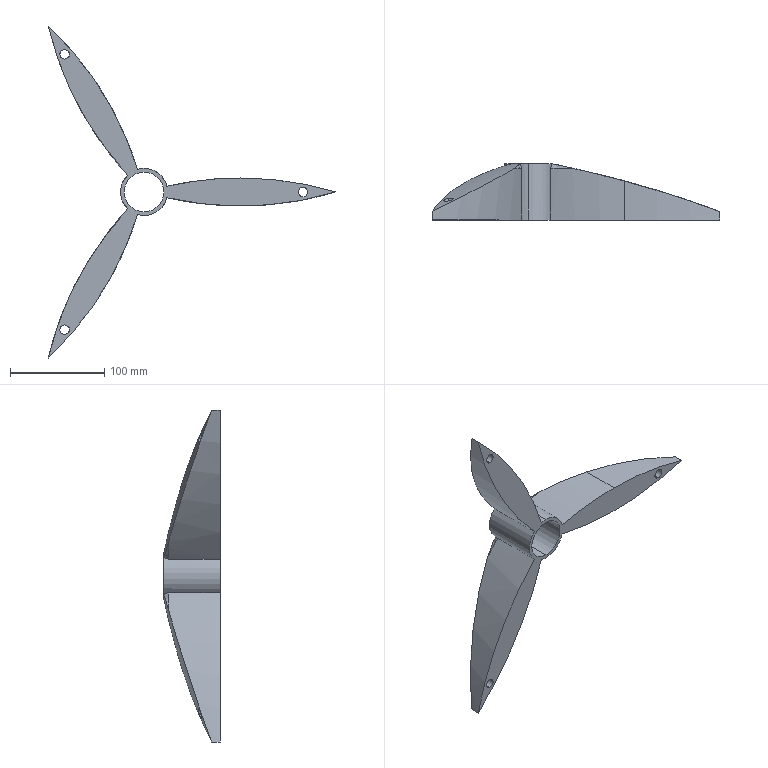Part | SolidWorks | features BaseBody 1 | 1 solid | 30 faces | box 305.237 x 60 x 352.457 mm | volume 492645 mm3 | cylinder 19 | spline 9 | plane 2 | commonest cylinder face diameters 700.36 x7 10.028 x6 50 x4 42.2 x2